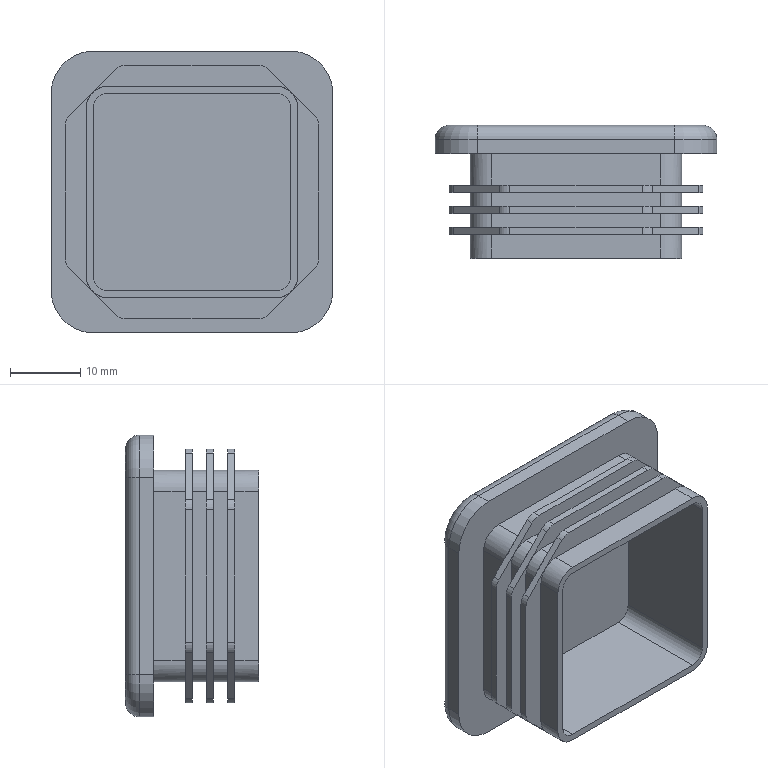Part | STEP file | 40方管堵头 | 1 solid | 132 faces | box 40 x 18.9 x 40 mm | volume 8663 mm3 | plane 76 | cylinder 52 | torus 4 | commonest cylinder face diameters 4 x32 6 x16 12 x4